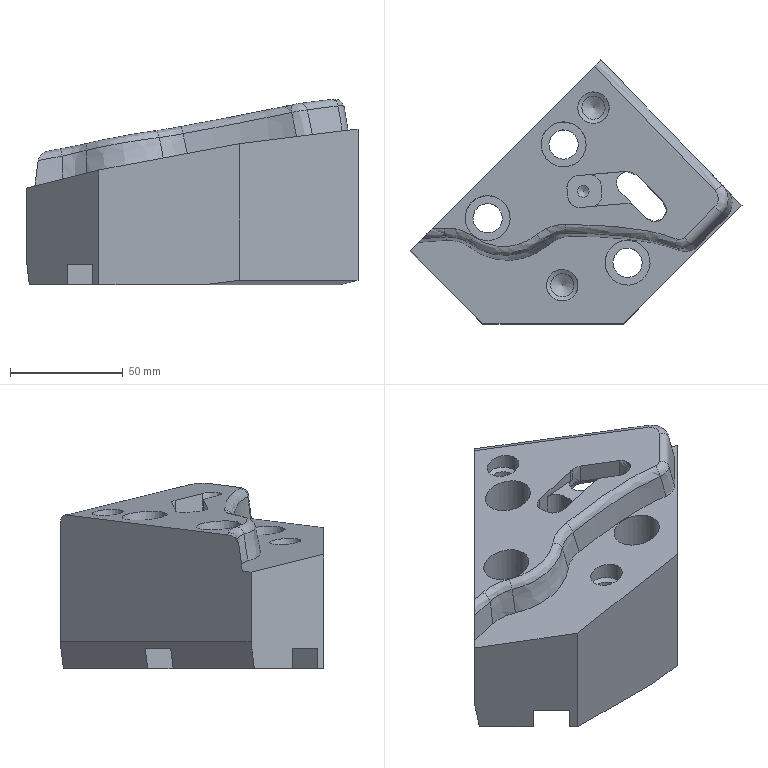Part | STEP file | 9805823380.1BPIECE_SOLIDE_FINALE_id370_x_t | 1 solid | 94 faces | box 147.437 x 117.174 x 82.369 mm | volume 503669 mm3 | plane 36 | spline 25 | cylinder 25 | cone 6 | other 2 | commonest cylinder face diameters 10.2 x5 8 x3 13 x3 14 x3 20 x3 10.3 x2